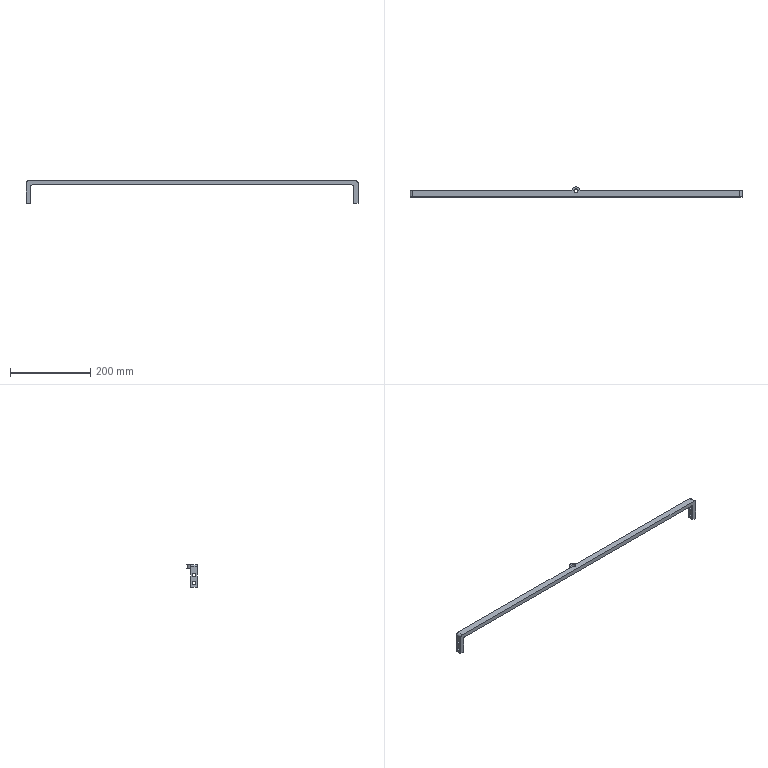Part | SolidWorks | features ICE 2, Extrusion 1, Fillet 1 | 1 solid | 26 faces | box 825 x 25 x 55 mm | volume 136025 mm3 | cylinder 15 | plane 11 | commonest cylinder face diameters 8 x8 10 x6 20 x1
STEP:
#1=CARTESIAN_POINT('',(-402.5,-7.5,-19.));
#2=VERTEX_POINT('',#1);
#3=CARTESIAN_POINT('',(-402.5,-7.5,-11.));
#4=VERTEX_POINT('',#3);
#5=CARTESIAN_POINT('',(-402.5,-7.5,-15.));
#6=DIRECTION('',(-1.,0.,0.));
#7=DIRECTION('',(0.,0.,1.));
#8=AXIS2_PLACEMENT_3D('',#5,#6,#7);
#9=CIRCLE('',#8,4.);
#10=EDGE_CURVE('',#2,#4,#9,.T.);
#11=ORIENTED_EDGE('',*,*,#10,.F.);
#12=CARTESIAN_POINT('',(-412.5,-7.5,-19.));
#13=VERTEX_POINT('',#12);
#14=CARTESIAN_POINT('',(-402.5,-7.5,-19.));
#15=DIRECTION('',(-1.,0.,0.));
#16=VECTOR('',#15,1000.);
#17=LINE('',#14,#16);
#18=EDGE_CURVE('',#2,#13,#17,.T.);
#19=ORIENTED_EDGE('',*,*,#18,.T.);
#20=CARTESIAN_POINT('',(-412.5,-7.5,-11.));
#21=VERTEX_POINT('',#20);
#22=CARTESIAN_POINT('',(-412.5,-7.5,-15.));
#23=DIRECTION('',(-1.,0.,0.));
#24=DIRECTION('',(0.,0.,1.));
#25=AXIS2_PLACEMENT_3D('',#22,#23,#24);
#26=CIRCLE('',#25,4.);
#27=EDGE_CURVE('',#13,#21,#26,.T.);
#28=ORIENTED_EDGE('',*,*,#27,.T.);
#29=CARTESIAN_POINT('',(-402.5,-7.5,-11.));
#30=DIRECTION('',(-1.,0.,0.));
#31=VECTOR('',#30,1000.);
#32=LINE('',#29,#31);
#33=EDGE_CURVE('',#4,#21,#32,.T.);
#34=ORIENTED_EDGE('',*,*,#33,.F.);
#35=EDGE_LOOP('',(#11,#19,#28,#34));
#36=FACE_OUTER_BOUND('',#35,.T.);
#37=CARTESIAN_POINT('',(-402.5,-7.5,-15.));
#38=DIRECTION('',(-1.,0.,0.));
#39=DIRECTION('',(0.,0.,1.));
#40=AXIS2_PLACEMENT_3D('',#37,#38,#39);
#41=CYLINDRICAL_SURFACE('',#40,4.);
#42=ADVANCED_FACE('',(#36),#41,.F.);
#43=CARTESIAN_POINT('',(-402.5,-7.5,-39.));
#44=VERTEX_POINT('',#43);
#45=CARTESIAN_POINT('',(-402.5,-7.5,-31.));
#46=VERTEX_POINT('',#45);
#47=CARTESIAN_POINT('',(-402.5,-7.5,-35.));
#48=DIRECTION('',(-1.,0.,0.));
#49=DIRECTION('',(0.,0.,1.));
#50=AXIS2_PLACEMENT_3D('',#47,#48,#49);
#51=CIRCLE('',#50,4.);
#52=EDGE_CURVE('',#44,#46,#51,.T.);
#53=ORIENTED_EDGE('',*,*,#52,.F.);
#54=CARTESIAN_POINT('',(-412.5,-7.5,-39.));
#55=VERTEX_POINT('',#54);
#56=CARTESIAN_POINT('',(-402.5,-7.5,-39.));
#57=DIRECTION('',(-1.,0.,0.));
#58=VECTOR('',#57,1000.);
#59=LINE('',#56,#58);
#60=EDGE_CURVE('',#44,#55,#59,.T.);
#61=ORIENTED_EDGE('',*,*,#60,.T.);
#62=CARTESIAN_POINT('',(-412.5,-7.5,-31.));
#63=VERTEX_POINT('',#62);
#64=CARTESIAN_POINT('',(-412.5,-7.5,-35.));
#65=DIRECTION('',(-1.,0.,0.));
#66=DIRECTION('',(0.,0.,1.));
#67=AXIS2_PLACEMENT_3D('',#64,#65,#66);
#68=CIRCLE('',#67,4.);
#69=EDGE_CURVE('',#55,#63,#68,.T.);
#70=ORIENTED_EDGE('',*,*,#69,.T.);
#71=CARTESIAN_POINT('',(-402.5,-7.5,-31.));
#72=DIRECTION('',(-1.,0.,0.));
#73=VECTOR('',#72,1000.);
#74=LINE('',#71,#73);
#75=EDGE_CURVE('',#46,#63,#74,.T.);
#76=ORIENTED_EDGE('',*,*,#75,.F.);
#77=EDGE_LOOP('',(#53,#61,#70,#76));
#78=FACE_OUTER_BOUND('',#77,.T.);
#79=CARTESIAN_POINT('',(-402.5,-7.5,-35.));
#80=DIRECTION('',(-1.,0.,0.));
#81=DIRECTION('',(0.,0.,1.));
#82=AXIS2_PLACEMENT_3D('',#79,#80,#81);
#83=CYLINDRICAL_SURFACE('',#82,4.);
#84=ADVANCED_FACE('',(#78),#83,.F.);
#85=CARTESIAN_POINT('',(402.5,-7.5,-31.));
#86=VERTEX_POINT('',#85);
#87=CARTESIAN_POINT('',(402.5,-7.5,-39.));
#88=VERTEX_POINT('',#87);
#89=CARTESIAN_POINT('',(402.5,-7.5,-35.));
#90=DIRECTION('',(1.,0.,0.));
#91=DIRECTION('',(0.,0.,-1.));
#92=AXIS2_PLACEMENT_3D('',#89,#90,#91);
#93=CIRCLE('',#92,4.);
#94=EDGE_CURVE('',#86,#88,#93,.T.);
#95=ORIENTED_EDGE('',*,*,#94,.F.);
#96=CARTESIAN_POINT('',(412.5,-7.5,-31.));
#97=VERTEX_POINT('',#96);
#98=CARTESIAN_POINT('',(402.5,-7.5,-31.));
#99=DIRECTION('',(1.,0.,0.));
#100=VECTOR('',#99,1000.);
#101=LINE('',#98,#100);
#102=EDGE_CURVE('',#86,#97,#101,.T.);
#103=ORIENTED_EDGE('',*,*,#102,.T.);
#104=CARTESIAN_POINT('',(412.5,-7.5,-39.));
#105=VERTEX_POINT('',#104);
#106=CARTESIAN_POINT('',(412.5,-7.5,-35.));
#107=DIRECTION('',(1.,0.,0.));
#108=DIRECTION('',(0.,0.,-1.));
#109=AXIS2_PLACEMENT_3D('',#106,#107,#108);
#110=CIRCLE('',#109,4.);
#111=EDGE_CURVE('',#97,#105,#110,.T.);
#112=ORIENTED_EDGE('',*,*,#111,.T.);
#113=CARTESIAN_POINT('',(402.5,-7.5,-39.));
#114=DIRECTION('',(1.,0.,0.));
#115=VECTOR('',#114,1000.);
#116=LINE('',#113,#115);
#117=EDGE_CURVE('',#88,#105,#116,.T.);
#118=ORIENTED_EDGE('',*,*,#117,.F.);
#119=EDGE_LOOP('',(#95,#103,#112,#118));
#120=FACE_OUTER_BOUND('',#119,.T.);
#121=CARTESIAN_POINT('',(402.5,-7.5,-35.));
#122=DIRECTION('',(1.,0.,0.));
#123=DIRECTION('',(0.,0.,-1.));
#124=AXIS2_PLACEMENT_3D('',#121,#122,#123);
#125=CYLINDRICAL_SURFACE('',#124,4.);
#126=ADVANCED_FACE('',(#120),#125,.F.);
#127=CARTESIAN_POINT('',(402.5,-7.5,-11.));
#128=VERTEX_POINT('',#127);
#129=CARTESIAN_POINT('',(402.5,-7.5,-19.));
#130=VERTEX_POINT('',#129);
#131=CARTESIAN_POINT('',(402.5,-7.5,-15.));
#132=DIRECTION('',(1.,0.,0.));
#133=DIRECTION('',(0.,0.,-1.));
#134=AXIS2_PLACEMENT_3D('',#131,#132,#133);
#135=CIRCLE('',#134,4.);
#136=EDGE_CURVE('',#128,#130,#135,.T.);
#137=ORIENTED_EDGE('',*,*,#136,.F.);
#138=CARTESIAN_POINT('',(412.5,-7.5,-11.));
#139=VERTEX_POINT('',#138);
#140=CARTESIAN_POINT('',(402.5,-7.5,-11.));
#141=DIRECTION('',(1.,0.,0.));
#142=VECTOR('',#141,1000.);
#143=LINE('',#140,#142);
#144=EDGE_CURVE('',#128,#139,#143,.T.);
#145=ORIENTED_EDGE('',*,*,#144,.T.);
#146=CARTESIAN_POINT('',(412.5,-7.5,-19.));
#147=VERTEX_POINT('',#146);
#148=CARTESIAN_POINT('',(412.5,-7.5,-15.));
#149=DIRECTION('',(1.,0.,0.));
#150=DIRECTION('',(0.,0.,-1.));
#151=AXIS2_PLACEMENT_3D('',#148,#149,#150);
#152=CIRCLE('',#151,4.);
#153=EDGE_CURVE('',#139,#147,#152,.T.);
#154=ORIENTED_EDGE('',*,*,#153,.T.);
#155=CARTESIAN_POINT('',(402.5,-7.5,-19.));
#156=DIRECTION('',(1.,0.,0.));
#157=VECTOR('',#156,1000.);
#158=LINE('',#155,#157);
#159=EDGE_CURVE('',#130,#147,#158,.T.);
#160=ORIENTED_EDGE('',*,*,#159,.F.);
#161=EDGE_LOOP('',(#137,#145,#154,#160));
#162=FACE_OUTER_BOUND('',#161,.T.);
#163=CARTESIAN_POINT('',(402.5,-7.5,-15.));
#164=DIRECTION('',(1.,0.,0.));
#165=DIRECTION('',(0.,0.,-1.));
#166=AXIS2_PLACEMENT_3D('',#163,#164,#165);
#167=CYLINDRICAL_SURFACE('',#166,4.);
#168=ADVANCED_FACE('',(#162),#167,.F.);
#169=CARTESIAN_POINT('',(-5.,0.,10.));
#170=VERTEX_POINT('',#169);
#171=CARTESIAN_POINT('',(5.,0.,10.));
#172=VERTEX_POINT('',#171);
#173=CARTESIAN_POINT('',(0.,0.,10.));
#174=DIRECTION('',(0.,0.,1.));
#175=DIRECTION('',(1.,0.,0.));
#176=AXIS2_PLACEMENT_3D('',#173,#174,#175);
#177=CIRCLE('',#176,5.);
#178=EDGE_CURVE('',#170,#172,#177,.T.);
#179=ORIENTED_EDGE('',*,*,#178,.T.);
#180=CARTESIAN_POINT('',(5.,0.,0.));
#181=VERTEX_POINT('',#180);
#182=CARTESIAN_POINT('',(5.,0.,10.));
#183=DIRECTION('',(0.,0.,-1.));
#184=VECTOR('',#183,1000.);
#185=LINE('',#182,#184);
#186=EDGE_CURVE('',#172,#181,#185,.T.);
#187=ORIENTED_EDGE('',*,*,#186,.T.);
#188=CARTESIAN_POINT('',(-5.,0.,0.));
#189=VERTEX_POINT('',#188);
#190=CARTESIAN_POINT('',(0.,0.,0.));
#191=DIRECTION('',(0.,0.,1.));
#192=DIRECTION('',(1.,0.,0.));
#193=AXIS2_PLACEMENT_3D('',#190,#191,#192);
#194=CIRCLE('',#193,5.);
#195=EDGE_CURVE('',#189,#181,#194,.T.);
#196=ORIENTED_EDGE('',*,*,#195,.F.);
#197=CARTESIAN_POINT('',(-5.,0.,10.));
#198=DIRECTION('',(0.,0.,-1.));
#199=VECTOR('',#198,1000.);
#200=LINE('',#197,#199);
#201=EDGE_CURVE('',#170,#189,#200,.T.);
#202=ORIENTED_EDGE('',*,*,#201,.F.);
#203=EDGE_LOOP('',(#179,#187,#196,#202));
#204=FACE_OUTER_BOUND('',#203,.T.);
#205=CARTESIAN_POINT('',(0.,0.,10.));
#206=DIRECTION('',(0.,0.,-1.));
#207=DIRECTION('',(-1.,0.,0.));
#208=AXIS2_PLACEMENT_3D('',#205,#206,#207);
#209=CYLINDRICAL_SURFACE('',#208,5.);
#210=ADVANCED_FACE('',(#204),#209,.F.);
#211=CARTESIAN_POINT('',(-10.,0.,10.));
#212=VERTEX_POINT('',#211);
#213=CARTESIAN_POINT('',(-407.5,0.,10.));
#214=VERTEX_POINT('',#213);
#215=CARTESIAN_POINT('',(-412.5,0.,10.));
#216=DIRECTION('',(-1.,0.,0.));
#217=VECTOR('',#216,1000.);
#218=LINE('',#215,#217);
#219=EDGE_CURVE('',#212,#214,#218,.T.);
#220=ORIENTED_EDGE('',*,*,#219,.T.);
#221=CARTESIAN_POINT('',(-407.5,-15.,10.));
#222=VERTEX_POINT('',#221);
#223=CARTESIAN_POINT('',(-407.5,-15.,10.));
#224=DIRECTION('',(0.,-1.,0.));
#225=VECTOR('',#224,1000.);
#226=LINE('',#223,#225);
#227=EDGE_CURVE('',#214,#222,#226,.T.);
#228=ORIENTED_EDGE('',*,*,#227,.T.);
#229=CARTESIAN_POINT('',(407.5,-15.,10.));
#230=VERTEX_POINT('',#229);
#231=CARTESIAN_POINT('',(0.,-15.,10.));
#232=DIRECTION('',(1.,0.,0.));
#233=VECTOR('',#232,1000.);
#234=LINE('',#231,#233);
#235=EDGE_CURVE('',#222,#230,#234,.T.);
#236=ORIENTED_EDGE('',*,*,#235,.T.);
#237=CARTESIAN_POINT('',(407.5,0.,10.));
#238=VERTEX_POINT('',#237);
#239=CARTESIAN_POINT('',(407.5,0.,10.));
#240=DIRECTION('',(0.,1.,0.));
#241=VECTOR('',#240,1000.);
#242=LINE('',#239,#241);
#243=EDGE_CURVE('',#230,#238,#242,.T.);
#244=ORIENTED_EDGE('',*,*,#243,.T.);
#245=CARTESIAN_POINT('',(10.,0.,10.));
#246=VERTEX_POINT('',#245);
#247=CARTESIAN_POINT('',(412.5,0.,10.));
#248=DIRECTION('',(-1.,0.,0.));
#249=VECTOR('',#248,1000.);
#250=LINE('',#247,#249);
#251=EDGE_CURVE('',#238,#246,#250,.T.);
#252=ORIENTED_EDGE('',*,*,#251,.T.);
#253=CARTESIAN_POINT('',(0.,0.,10.));
#254=DIRECTION('',(0.,0.,1.));
#255=DIRECTION('',(1.,0.,0.));
#256=AXIS2_PLACEMENT_3D('',#253,#254,#255);
#257=CIRCLE('',#256,10.);
#258=EDGE_CURVE('',#246,#212,#257,.T.);
#259=ORIENTED_EDGE('',*,*,#258,.T.);
#260=EDGE_LOOP('',(#220,#228,#236,#244,#252,#259));
#261=FACE_OUTER_BOUND('',#260,.T.);
#262=ORIENTED_EDGE('',*,*,#178,.F.);
#263=CARTESIAN_POINT('',(0.,0.,10.));
#264=DIRECTION('',(0.,0.,1.));
#265=DIRECTION('',(1.,0.,0.));
#266=AXIS2_PLACEMENT_3D('',#263,#264,#265);
#267=CIRCLE('',#266,5.);
#268=EDGE_CURVE('',#172,#170,#267,.T.);
#269=ORIENTED_EDGE('',*,*,#268,.F.);
#270=EDGE_LOOP('',(#262,#269));
#271=FACE_BOUND('',#270,.T.);
#272=CARTESIAN_POINT('',(0.,0.,10.));
#273=DIRECTION('',(0.,0.,1.));
#274=DIRECTION('',(1.,0.,0.));
#275=AXIS2_PLACEMENT_3D('',#272,#273,#274);
#276=PLANE('',#275);
#277=ADVANCED_FACE('',(#261,#271),#276,.T.);
#278=CARTESIAN_POINT('',(397.5,0.,0.));
#279=VERTEX_POINT('',#278);
#280=CARTESIAN_POINT('',(10.,0.,0.));
#281=VERTEX_POINT('',#280);
#282=CARTESIAN_POINT('',(412.5,0.,0.));
#283=DIRECTION('',(-1.,0.,0.));
#284=VECTOR('',#283,1000.);
#285=LINE('',#282,#284);
#286=EDGE_CURVE('',#279,#281,#285,.T.);
#287=ORIENTED_EDGE('',*,*,#286,.F.);
#288=CARTESIAN_POINT('',(397.5,-15.,0.));
#289=VERTEX_POINT('',#288);
#290=CARTESIAN_POINT('',(397.5,-15.,0.));
#291=DIRECTION('',(0.,-1.,0.));
#292=VECTOR('',#291,1000.);
#293=LINE('',#290,#292);
#294=EDGE_CURVE('',#279,#289,#293,.T.);
#295=ORIENTED_EDGE('',*,*,#294,.T.);
#296=CARTESIAN_POINT('',(-397.5,-15.,0.));
#297=VERTEX_POINT('',#296);
#298=CARTESIAN_POINT('',(0.,-15.,0.));
#299=DIRECTION('',(1.,0.,0.));
#300=VECTOR('',#299,1000.);
#301=LINE('',#298,#300);
#302=EDGE_CURVE('',#297,#289,#301,.T.);
#303=ORIENTED_EDGE('',*,*,#302,.F.);
#304=CARTESIAN_POINT('',(-397.5,0.,0.));
#305=VERTEX_POINT('',#304);
#306=CARTESIAN_POINT('',(-397.5,0.,0.));
#307=DIRECTION('',(0.,1.,0.));
#308=VECTOR('',#307,1000.);
#309=LINE('',#306,#308);
#310=EDGE_CURVE('',#297,#305,#309,.T.);
#311=ORIENTED_EDGE('',*,*,#310,.T.);
#312=CARTESIAN_POINT('',(-10.,0.,0.));
#313=VERTEX_POINT('',#312);
#314=CARTESIAN_POINT('',(-412.5,0.,0.));
#315=DIRECTION('',(-1.,0.,0.));
#316=VECTOR('',#315,1000.);
#317=LINE('',#314,#316);
#318=EDGE_CURVE('',#313,#305,#317,.T.);
#319=ORIENTED_EDGE('',*,*,#318,.F.);
#320=CARTESIAN_POINT('',(0.,0.,0.));
#321=DIRECTION('',(0.,0.,1.));
#322=DIRECTION('',(1.,0.,0.));
#323=AXIS2_PLACEMENT_3D('',#320,#321,#322);
#324=CIRCLE('',#323,10.);
#325=EDGE_CURVE('',#281,#313,#324,.T.);
#326=ORIENTED_EDGE('',*,*,#325,.F.);
#327=EDGE_LOOP('',(#287,#295,#303,#311,#319,#326));
#328=FACE_OUTER_BOUND('',#327,.T.);
#329=ORIENTED_EDGE('',*,*,#195,.T.);
#330=CARTESIAN_POINT('',(0.,0.,0.));
#331=DIRECTION('',(0.,0.,1.));
#332=DIRECTION('',(1.,0.,0.));
#333=AXIS2_PLACEMENT_3D('',#330,#331,#332);
#334=CIRCLE('',#333,5.);
#335=EDGE_CURVE('',#181,#189,#334,.T.);
#336=ORIENTED_EDGE('',*,*,#335,.T.);
#337=EDGE_LOOP('',(#329,#336));
#338=FACE_BOUND('',#337,.T.);
#339=CARTESIAN_POINT('',(0.,0.,0.));
#340=DIRECTION('',(0.,0.,1.));
#341=DIRECTION('',(1.,0.,0.));
#342=AXIS2_PLACEMENT_3D('',#339,#340,#341);
#343=PLANE('',#342);
#344=ADVANCED_FACE('',(#328,#338),#343,.F.);
#345=ORIENTED_EDGE('',*,*,#251,.F.);
#346=CARTESIAN_POINT('',(412.5,0.,5.));
#347=VERTEX_POINT('',#346);
#348=CARTESIAN_POINT('',(407.5,0.,5.));
#349=DIRECTION('',(0.,1.,0.));
#350=DIRECTION('',(0.,0.,-1.));
#351=AXIS2_PLACEMENT_3D('',#348,#349,#350);
#352=CIRCLE('',#351,5.);
#353=EDGE_CURVE('',#238,#347,#352,.T.);
#354=ORIENTED_EDGE('',*,*,#353,.T.);
#355=CARTESIAN_POINT('',(412.5,0.,-45.));
#356=VERTEX_POINT('',#355);
#357=CARTESIAN_POINT('',(412.5,0.,10.));
#358=DIRECTION('',(0.,0.,-1.));
#359=VECTOR('',#358,1000.);
#360=LINE('',#357,#359);
#361=EDGE_CURVE('',#347,#356,#360,.T.);
#362=ORIENTED_EDGE('',*,*,#361,.T.);
#363=CARTESIAN_POINT('',(402.5,0.,-45.));
#364=VERTEX_POINT('',#363);
#365=CARTESIAN_POINT('',(402.5,0.,-45.));
#366=DIRECTION('',(1.,0.,0.));
#367=VECTOR('',#366,1000.);
#368=LINE('',#365,#367);
#369=EDGE_CURVE('',#364,#356,#368,.T.);
#370=ORIENTED_EDGE('',*,*,#369,.F.);
#371=CARTESIAN_POINT('',(402.5,0.,-5.));
#372=VERTEX_POINT('',#371);
#373=CARTESIAN_POINT('',(402.5,0.,0.));
#374=DIRECTION('',(0.,0.,1.));
#375=VECTOR('',#374,1000.);
#376=LINE('',#373,#375);
#377=EDGE_CURVE('',#364,#372,#376,.T.);
#378=ORIENTED_EDGE('',*,*,#377,.T.);
#379=CARTESIAN_POINT('',(397.5,0.,-5.));
#380=DIRECTION('',(0.,-1.,0.));
#381=DIRECTION('',(0.,0.,-1.));
#382=AXIS2_PLACEMENT_3D('',#379,#380,#381);
#383=CIRCLE('',#382,5.);
#384=EDGE_CURVE('',#372,#279,#383,.T.);
#385=ORIENTED_EDGE('',*,*,#384,.T.);
#386=ORIENTED_EDGE('',*,*,#286,.T.);
#387=CARTESIAN_POINT('',(10.,0.,10.));
#388=DIRECTION('',(0.,0.,-1.));
#389=VECTOR('',#388,1000.);
#390=LINE('',#387,#389);
#391=EDGE_CURVE('',#246,#281,#390,.T.);
#392=ORIENTED_EDGE('',*,*,#391,.F.);
#393=EDGE_LOOP('',(#345,#354,#362,#370,#378,#385,#386,#392));
#394=FACE_OUTER_BOUND('',#393,.T.);
#395=CARTESIAN_POINT('',(412.5,0.,10.));
#396=DIRECTION('',(0.,-1.,0.));
#397=DIRECTION('',(0.,0.,-1.));
#398=AXIS2_PLACEMENT_3D('',#395,#396,#397);
#399=PLANE('',#398);
#400=ADVANCED_FACE('',(#394),#399,.F.);
#401=ORIENTED_EDGE('',*,*,#325,.T.);
#402=CARTESIAN_POINT('',(-10.,0.,10.));
#403=DIRECTION('',(0.,0.,-1.));
#404=VECTOR('',#403,1000.);
#405=LINE('',#402,#404);
#406=EDGE_CURVE('',#212,#313,#405,.T.);
#407=ORIENTED_EDGE('',*,*,#406,.F.);
#408=ORIENTED_EDGE('',*,*,#258,.F.);
#409=ORIENTED_EDGE('',*,*,#391,.T.);
#410=EDGE_LOOP('',(#401,#407,#408,#409));
#411=FACE_OUTER_BOUND('',#410,.T.);
#412=CARTESIAN_POINT('',(0.,0.,10.));
#413=DIRECTION('',(0.,0.,-1.));
#414=DIRECTION('',(-1.,0.,0.));
#415=AXIS2_PLACEMENT_3D('',#412,#413,#414);
#416=CYLINDRICAL_SURFACE('',#415,10.);
#417=ADVANCED_FACE('',(#411),#416,.T.);
#418=CARTESIAN_POINT('',(-412.5,0.,5.));
#419=VERTEX_POINT('',#418);
#420=CARTESIAN_POINT('',(-412.5,0.,-45.));
#421=VERTEX_POINT('',#420);
#422=CARTESIAN_POINT('',(-412.5,0.,10.));
#423=DIRECTION('',(0.,0.,-1.));
#424=VECTOR('',#423,1000.);
#425=LINE('',#422,#424);
#426=EDGE_CURVE('',#419,#421,#425,.T.);
#427=ORIENTED_EDGE('',*,*,#426,.F.);
#428=CARTESIAN_POINT('',(-407.5,0.,5.));
#429=DIRECTION('',(0.,1.,0.));
#430=DIRECTION('',(0.,0.,-1.));
#431=AXIS2_PLACEMENT_3D('',#428,#429,#430);
#432=CIRCLE('',#431,5.);
#433=EDGE_CURVE('',#419,#214,#432,.T.);
#434=ORIENTED_EDGE('',*,*,#433,.T.);
#435=ORIENTED_EDGE('',*,*,#219,.F.);
#436=ORIENTED_EDGE('',*,*,#406,.T.);
#437=ORIENTED_EDGE('',*,*,#318,.T.);
#438=CARTESIAN_POINT('',(-402.5,0.,-5.));
#439=VERTEX_POINT('',#438);
#440=CARTESIAN_POINT('',(-397.5,0.,-5.));
#441=DIRECTION('',(0.,-1.,0.));
#442=DIRECTION('',(0.,0.,-1.));
#443=AXIS2_PLACEMENT_3D('',#440,#441,#442);
#444=CIRCLE('',#443,5.);
#445=EDGE_CURVE('',#305,#439,#444,.T.);
#446=ORIENTED_EDGE('',*,*,#445,.T.);
#447=CARTESIAN_POINT('',(-402.5,0.,-45.));
#448=VERTEX_POINT('',#447);
#449=CARTESIAN_POINT('',(-402.5,0.,0.));
#450=DIRECTION('',(0.,0.,-1.));
#451=VECTOR('',#450,1000.);
#452=LINE('',#449,#451);
#453=EDGE_CURVE('',#439,#448,#452,.T.);
#454=ORIENTED_EDGE('',*,*,#453,.T.);
#455=CARTESIAN_POINT('',(-402.5,0.,-45.));
#456=DIRECTION('',(-1.,0.,0.));
#457=VECTOR('',#456,1000.);
#458=LINE('',#455,#457);
#459=EDGE_CURVE('',#448,#421,#458,.T.);
#460=ORIENTED_EDGE('',*,*,#459,.T.);
#461=EDGE_LOOP('',(#427,#434,#435,#436,#437,#446,#454,#460));
#462=FACE_OUTER_BOUND('',#461,.T.);
#463=CARTESIAN_POINT('',(-412.5,0.,10.));
#464=DIRECTION('',(0.,-1.,0.));
#465=DIRECTION('',(0.,0.,-1.));
#466=AXIS2_PLACEMENT_3D('',#463,#464,#465);
#467=PLANE('',#466);
#468=ADVANCED_FACE('',(#462),#467,.F.);
#469=CARTESIAN_POINT('',(-412.5,-15.,5.));
#470=VERTEX_POINT('',#469);
#471=CARTESIAN_POINT('',(-412.5,-15.,-45.));
#472=VERTEX_POINT('',#471);
#473=CARTESIAN_POINT('',(-412.5,-15.,10.));
#474=DIRECTION('',(0.,0.,-1.));
#475=VECTOR('',#474,1000.);
#476=LINE('',#473,#475);
#477=EDGE_CURVE('',#470,#472,#476,.T.);
#478=ORIENTED_EDGE('',*,*,#477,.F.);
#479=CARTESIAN_POINT('',(-412.5,0.,5.));
#480=DIRECTION('',(0.,1.,0.));
#481=VECTOR('',#480,1000.);
#482=LINE('',#479,#481);
#483=EDGE_CURVE('',#470,#419,#482,.T.);
#484=ORIENTED_EDGE('',*,*,#483,.T.);
#485=ORIENTED_EDGE('',*,*,#426,.T.);
#486=CARTESIAN_POINT('',(-412.5,0.,-45.));
#487=DIRECTION('',(0.,-1.,0.));
#488=VECTOR('',#487,1000.);
#489=LINE('',#486,#488);
#490=EDGE_CURVE('',#421,#472,#489,.T.);
#491=ORIENTED_EDGE('',*,*,#490,.T.);
#492=EDGE_LOOP('',(#478,#484,#485,#491));
#493=FACE_OUTER_BOUND('',#492,.T.);
#494=CARTESIAN_POINT('',(-412.5,-7.5,-15.));
#495=DIRECTION('',(-1.,0.,0.));
#496=DIRECTION('',(0.,0.,1.));
#497=AXIS2_PLACEMENT_3D('',#494,#495,#496);
#498=CIRCLE('',#497,4.);
#499=EDGE_CURVE('',#21,#13,#498,.T.);
#500=ORIENTED_EDGE('',*,*,#499,.F.);
#501=ORIENTED_EDGE('',*,*,#27,.F.);
#502=EDGE_LOOP('',(#500,#501));
#503=FACE_BOUND('',#502,.T.);
#504=CARTESIAN_POINT('',(-412.5,-7.5,-35.));
#505=DIRECTION('',(-1.,0.,0.));
#506=DIRECTION('',(0.,0.,1.));
#507=AXIS2_PLACEMENT_3D('',#504,#505,#506);
#508=CIRCLE('',#507,4.);
#509=EDGE_CURVE('',#63,#55,#508,.T.);
#510=ORIENTED_EDGE('',*,*,#509,.F.);
#511=ORIENTED_EDGE('',*,*,#69,.F.);
#512=EDGE_LOOP('',(#510,#511));
#513=FACE_BOUND('',#512,.T.);
#514=CARTESIAN_POINT('',(-412.5,-15.,10.));
#515=DIRECTION('',(1.,0.,0.));
#516=DIRECTION('',(0.,0.,-1.));
#517=AXIS2_PLACEMENT_3D('',#514,#515,#516);
#518=PLANE('',#517);
#519=ADVANCED_FACE('',(#493,#503,#513),#518,.F.);
#520=ORIENTED_EDGE('',*,*,#235,.F.);
#521=CARTESIAN_POINT('',(-407.5,-15.,5.));
#522=DIRECTION('',(0.,-1.,0.));
#523=DIRECTION('',(0.,0.,1.));
#524=AXIS2_PLACEMENT_3D('',#521,#522,#523);
#525=CIRCLE('',#524,5.);
#526=EDGE_CURVE('',#222,#470,#525,.T.);
#527=ORIENTED_EDGE('',*,*,#526,.T.);
#528=ORIENTED_EDGE('',*,*,#477,.T.);
#529=CARTESIAN_POINT('',(-402.5,-15.,-45.));
#530=VERTEX_POINT('',#529);
#531=CARTESIAN_POINT('',(-402.5,-15.,-45.));
#532=DIRECTION('',(-1.,0.,0.));
#533=VECTOR('',#532,1000.);
#534=LINE('',#531,#533);
#535=EDGE_CURVE('',#530,#472,#534,.T.);
#536=ORIENTED_EDGE('',*,*,#535,.F.);
#537=CARTESIAN_POINT('',(-402.5,-15.,-5.));
#538=VERTEX_POINT('',#537);
#539=CARTESIAN_POINT('',(-402.5,-15.,0.));
#540=DIRECTION('',(0.,0.,1.));
#541=VECTOR('',#540,1000.);
#542=LINE('',#539,#541);
#543=EDGE_CURVE('',#530,#538,#542,.T.);
#544=ORIENTED_EDGE('',*,*,#543,.T.);
#545=CARTESIAN_POINT('',(-397.5,-15.,-5.));
#546=DIRECTION('',(0.,1.,0.));
#547=DIRECTION('',(0.,0.,1.));
#548=AXIS2_PLACEMENT_3D('',#545,#546,#547);
#549=CIRCLE('',#548,5.);
#550=EDGE_CURVE('',#538,#297,#549,.T.);
#551=ORIENTED_EDGE('',*,*,#550,.T.);
#552=ORIENTED_EDGE('',*,*,#302,.T.);
#553=CARTESIAN_POINT('',(402.5,-15.,-5.));
#554=VERTEX_POINT('',#553);
#555=CARTESIAN_POINT('',(397.5,-15.,-5.));
#556=DIRECTION('',(0.,1.,0.));
#557=DIRECTION('',(0.,0.,1.));
#558=AXIS2_PLACEMENT_3D('',#555,#556,#557);
#559=CIRCLE('',#558,5.);
#560=EDGE_CURVE('',#289,#554,#559,.T.);
#561=ORIENTED_EDGE('',*,*,#560,.T.);
#562=CARTESIAN_POINT('',(402.5,-15.,-45.));
#563=VERTEX_POINT('',#562);
#564=CARTESIAN_POINT('',(402.5,-15.,0.));
#565=DIRECTION('',(0.,0.,-1.));
#566=VECTOR('',#565,1000.);
#567=LINE('',#564,#566);
#568=EDGE_CURVE('',#554,#563,#567,.T.);
#569=ORIENTED_EDGE('',*,*,#568,.T.);
#570=CARTESIAN_POINT('',(412.5,-15.,-45.));
#571=VERTEX_POINT('',#570);
#572=CARTESIAN_POINT('',(402.5,-15.,-45.));
#573=DIRECTION('',(1.,0.,0.));
#574=VECTOR('',#573,1000.);
#575=LINE('',#572,#574);
#576=EDGE_CURVE('',#563,#571,#575,.T.);
#577=ORIENTED_EDGE('',*,*,#576,.T.);
#578=CARTESIAN_POINT('',(412.5,-15.,5.));
#579=VERTEX_POINT('',#578);
#580=CARTESIAN_POINT('',(412.5,-15.,10.));
#581=DIRECTION('',(0.,0.,-1.));
#582=VECTOR('',#581,1000.);
#583=LINE('',#580,#582);
#584=EDGE_CURVE('',#579,#571,#583,.T.);
#585=ORIENTED_EDGE('',*,*,#584,.F.);
#586=CARTESIAN_POINT('',(407.5,-15.,5.));
#587=DIRECTION('',(0.,-1.,0.));
#588=DIRECTION('',(0.,0.,1.));
#589=AXIS2_PLACEMENT_3D('',#586,#587,#588);
#590=CIRCLE('',#589,5.);
#591=EDGE_CURVE('',#579,#230,#590,.T.);
#592=ORIENTED_EDGE('',*,*,#591,.T.);
#593=EDGE_LOOP('',(#520,#527,#528,#536,#544,#551,#552,#561,#569,#577,#585,#592));
#594=FACE_OUTER_BOUND('',#593,.T.);
#595=CARTESIAN_POINT('',(0.,-15.,10.));
#596=DIRECTION('',(0.,1.,0.));
#597=DIRECTION('',(0.,0.,1.));
#598=AXIS2_PLACEMENT_3D('',#595,#596,#597);
#599=PLANE('',#598);
#600=ADVANCED_FACE('',(#594),#599,.F.);
#601=ORIENTED_EDGE('',*,*,#361,.F.);
#602=CARTESIAN_POINT('',(412.5,-15.,5.));
#603=DIRECTION('',(0.,-1.,0.));
#604=VECTOR('',#603,1000.);
#605=LINE('',#602,#604);
#606=EDGE_CURVE('',#347,#579,#605,.T.);
#607=ORIENTED_EDGE('',*,*,#606,.T.);
#608=ORIENTED_EDGE('',*,*,#584,.T.);
#609=CARTESIAN_POINT('',(412.5,0.,-45.));
#610=DIRECTION('',(0.,1.,0.));
#611=VECTOR('',#610,1000.);
#612=LINE('',#609,#611);
#613=EDGE_CURVE('',#571,#356,#612,.T.);
#614=ORIENTED_EDGE('',*,*,#613,.T.);
#615=EDGE_LOOP('',(#601,#607,#608,#614));
#616=FACE_OUTER_BOUND('',#615,.T.);
#617=CARTESIAN_POINT('',(412.5,-7.5,-35.));
#618=DIRECTION('',(1.,0.,0.));
#619=DIRECTION('',(0.,0.,-1.));
#620=AXIS2_PLACEMENT_3D('',#617,#618,#619);
#621=CIRCLE('',#620,4.);
#622=EDGE_CURVE('',#105,#97,#621,.T.);
#623=ORIENTED_EDGE('',*,*,#622,.F.);
#624=ORIENTED_EDGE('',*,*,#111,.F.);
#625=EDGE_LOOP('',(#623,#624));
#626=FACE_BOUND('',#625,.T.);
#627=CARTESIAN_POINT('',(412.5,-7.5,-15.));
#628=DIRECTION('',(1.,0.,0.));
#629=DIRECTION('',(0.,0.,-1.));
#630=AXIS2_PLACEMENT_3D('',#627,#628,#629);
#631=CIRCLE('',#630,4.);
#632=EDGE_CURVE('',#147,#139,#631,.T.);
#633=ORIENTED_EDGE('',*,*,#632,.F.);
#634=ORIENTED_EDGE('',*,*,#153,.F.);
#635=EDGE_LOOP('',(#633,#634));
#636=FACE_BOUND('',#635,.T.);
#637=CARTESIAN_POINT('',(412.5,-15.,10.));
#638=DIRECTION('',(-1.,0.,0.));
#639=DIRECTION('',(0.,0.,1.));
#640=AXIS2_PLACEMENT_3D('',#637,#638,#639);
#641=PLANE('',#640);
#642=ADVANCED_FACE('',(#616,#626,#636),#641,.F.);
#643=ORIENTED_EDGE('',*,*,#186,.F.);
#644=ORIENTED_EDGE('',*,*,#268,.T.);
#645=ORIENTED_EDGE('',*,*,#201,.T.);
#646=ORIENTED_EDGE('',*,*,#335,.F.);
#647=EDGE_LOOP('',(#643,#644,#645,#646));
#648=FACE_OUTER_BOUND('',#647,.T.);
#649=CARTESIAN_POINT('',(0.,0.,10.));
#650=DIRECTION('',(0.,0.,-1.));
#651=DIRECTION('',(-1.,0.,0.));
#652=AXIS2_PLACEMENT_3D('',#649,#650,#651);
#653=CYLINDRICAL_SURFACE('',#652,5.);
#654=ADVANCED_FACE('',(#648),#653,.F.);
#655=ORIENTED_EDGE('',*,*,#613,.F.);
#656=ORIENTED_EDGE('',*,*,#576,.F.);
#657=CARTESIAN_POINT('',(402.5,0.,-45.));
#658=DIRECTION('',(0.,1.,0.));
#659=VECTOR('',#658,1000.);
#660=LINE('',#657,#659);
#661=EDGE_CURVE('',#563,#364,#660,.T.);
#662=ORIENTED_EDGE('',*,*,#661,.T.);
#663=ORIENTED_EDGE('',*,*,#369,.T.);
#664=EDGE_LOOP('',(#655,#656,#662,#663));
#665=FACE_OUTER_BOUND('',#664,.T.);
#666=CARTESIAN_POINT('',(402.5,0.,-45.));
#667=DIRECTION('',(0.,0.,-1.));
#668=DIRECTION('',(-1.,0.,0.));
#669=AXIS2_PLACEMENT_3D('',#666,#667,#668);
#670=PLANE('',#669);
#671=ADVANCED_FACE('',(#665),#670,.T.);
#672=CARTESIAN_POINT('',(402.5,-7.5,-35.));
#673=DIRECTION('',(1.,0.,0.));
#674=DIRECTION('',(0.,0.,-1.));
#675=AXIS2_PLACEMENT_3D('',#672,#673,#674);
#676=CIRCLE('',#675,4.);
#677=EDGE_CURVE('',#88,#86,#676,.T.);
#678=ORIENTED_EDGE('',*,*,#677,.T.);
#679=ORIENTED_EDGE('',*,*,#94,.T.);
#680=EDGE_LOOP('',(#678,#679));
#681=FACE_BOUND('',#680,.T.);
#682=CARTESIAN_POINT('',(402.5,-7.5,-15.));
#683=DIRECTION('',(1.,0.,0.));
#684=DIRECTION('',(0.,0.,-1.));
#685=AXIS2_PLACEMENT_3D('',#682,#683,#684);
#686=CIRCLE('',#685,4.);
#687=EDGE_CURVE('',#130,#128,#686,.T.);
#688=ORIENTED_EDGE('',*,*,#687,.T.);
#689=ORIENTED_EDGE('',*,*,#136,.T.);
#690=EDGE_LOOP('',(#688,#689));
#691=FACE_BOUND('',#690,.T.);
#692=ORIENTED_EDGE('',*,*,#568,.F.);
#693=CARTESIAN_POINT('',(402.5,0.,-5.));
#694=DIRECTION('',(0.,1.,0.));
#695=VECTOR('',#694,1000.);
#696=LINE('',#693,#695);
#697=EDGE_CURVE('',#554,#372,#696,.T.);
#698=ORIENTED_EDGE('',*,*,#697,.T.);
#699=ORIENTED_EDGE('',*,*,#377,.F.);
#700=ORIENTED_EDGE('',*,*,#661,.F.);
#701=EDGE_LOOP('',(#692,#698,#699,#700));
#702=FACE_OUTER_BOUND('',#701,.T.);
#703=CARTESIAN_POINT('',(402.5,0.,0.));
#704=DIRECTION('',(1.,0.,0.));
#705=DIRECTION('',(0.,0.,-1.));
#706=AXIS2_PLACEMENT_3D('',#703,#704,#705);
#707=PLANE('',#706);
#708=ADVANCED_FACE('',(#681,#691,#702),#707,.F.);
#709=ORIENTED_EDGE('',*,*,#144,.F.);
#710=ORIENTED_EDGE('',*,*,#687,.F.);
#711=ORIENTED_EDGE('',*,*,#159,.T.);
#712=ORIENTED_EDGE('',*,*,#632,.T.);
#713=EDGE_LOOP('',(#709,#710,#711,#712));
#714=FACE_OUTER_BOUND('',#713,.T.);
#715=CARTESIAN_POINT('',(402.5,-7.5,-15.));
#716=DIRECTION('',(1.,0.,0.));
#717=DIRECTION('',(0.,0.,-1.));
#718=AXIS2_PLACEMENT_3D('',#715,#716,#717);
#719=CYLINDRICAL_SURFACE('',#718,4.);
#720=ADVANCED_FACE('',(#714),#719,.F.);
#721=ORIENTED_EDGE('',*,*,#102,.F.);
#722=ORIENTED_EDGE('',*,*,#677,.F.);
#723=ORIENTED_EDGE('',*,*,#117,.T.);
#724=ORIENTED_EDGE('',*,*,#622,.T.);
#725=EDGE_LOOP('',(#721,#722,#723,#724));
#726=FACE_OUTER_BOUND('',#725,.T.);
#727=CARTESIAN_POINT('',(402.5,-7.5,-35.));
#728=DIRECTION('',(1.,0.,0.));
#729=DIRECTION('',(0.,0.,-1.));
#730=AXIS2_PLACEMENT_3D('',#727,#728,#729);
#731=CYLINDRICAL_SURFACE('',#730,4.);
#732=ADVANCED_FACE('',(#726),#731,.F.);
#733=ORIENTED_EDGE('',*,*,#490,.F.);
#734=ORIENTED_EDGE('',*,*,#459,.F.);
#735=CARTESIAN_POINT('',(-402.5,0.,-45.));
#736=DIRECTION('',(0.,-1.,0.));
#737=VECTOR('',#736,1000.);
#738=LINE('',#735,#737);
#739=EDGE_CURVE('',#448,#530,#738,.T.);
#740=ORIENTED_EDGE('',*,*,#739,.T.);
#741=ORIENTED_EDGE('',*,*,#535,.T.);
#742=EDGE_LOOP('',(#733,#734,#740,#741));
#743=FACE_OUTER_BOUND('',#742,.T.);
#744=CARTESIAN_POINT('',(-402.5,0.,-45.));
#745=DIRECTION('',(0.,0.,-1.));
#746=DIRECTION('',(-1.,0.,0.));
#747=AXIS2_PLACEMENT_3D('',#744,#745,#746);
#748=PLANE('',#747);
#749=ADVANCED_FACE('',(#743),#748,.T.);
#750=CARTESIAN_POINT('',(-402.5,-7.5,-15.));
#751=DIRECTION('',(-1.,0.,0.));
#752=DIRECTION('',(0.,0.,1.));
#753=AXIS2_PLACEMENT_3D('',#750,#751,#752);
#754=CIRCLE('',#753,4.);
#755=EDGE_CURVE('',#4,#2,#754,.T.);
#756=ORIENTED_EDGE('',*,*,#755,.T.);
#757=ORIENTED_EDGE('',*,*,#10,.T.);
#758=EDGE_LOOP('',(#756,#757));
#759=FACE_BOUND('',#758,.T.);
#760=CARTESIAN_POINT('',(-402.5,-7.5,-35.));
#761=DIRECTION('',(-1.,0.,0.));
#762=DIRECTION('',(0.,0.,1.));
#763=AXIS2_PLACEMENT_3D('',#760,#761,#762);
#764=CIRCLE('',#763,4.);
#765=EDGE_CURVE('',#46,#44,#764,.T.);
#766=ORIENTED_EDGE('',*,*,#765,.T.);
#767=ORIENTED_EDGE('',*,*,#52,.T.);
#768=EDGE_LOOP('',(#766,#767));
#769=FACE_BOUND('',#768,.T.);
#770=ORIENTED_EDGE('',*,*,#453,.F.);
#771=CARTESIAN_POINT('',(-402.5,0.,-5.));
#772=DIRECTION('',(0.,-1.,0.));
#773=VECTOR('',#772,1000.);
#774=LINE('',#771,#773);
#775=EDGE_CURVE('',#439,#538,#774,.T.);
#776=ORIENTED_EDGE('',*,*,#775,.T.);
#777=ORIENTED_EDGE('',*,*,#543,.F.);
#778=ORIENTED_EDGE('',*,*,#739,.F.);
#779=EDGE_LOOP('',(#770,#776,#777,#778));
#780=FACE_OUTER_BOUND('',#779,.T.);
#781=CARTESIAN_POINT('',(-402.5,0.,0.));
#782=DIRECTION('',(1.,0.,0.));
#783=DIRECTION('',(0.,0.,-1.));
#784=AXIS2_PLACEMENT_3D('',#781,#782,#783);
#785=PLANE('',#784);
#786=ADVANCED_FACE('',(#759,#769,#780),#785,.T.);
#787=ORIENTED_EDGE('',*,*,#60,.F.);
#788=ORIENTED_EDGE('',*,*,#765,.F.);
#789=ORIENTED_EDGE('',*,*,#75,.T.);
#790=ORIENTED_EDGE('',*,*,#509,.T.);
#791=EDGE_LOOP('',(#787,#788,#789,#790));
#792=FACE_OUTER_BOUND('',#791,.T.);
#793=CARTESIAN_POINT('',(-402.5,-7.5,-35.));
#794=DIRECTION('',(-1.,0.,0.));
#795=DIRECTION('',(0.,0.,1.));
#796=AXIS2_PLACEMENT_3D('',#793,#794,#795);
#797=CYLINDRICAL_SURFACE('',#796,4.);
#798=ADVANCED_FACE('',(#792),#797,.F.);
#799=ORIENTED_EDGE('',*,*,#18,.F.);
#800=ORIENTED_EDGE('',*,*,#755,.F.);
#801=ORIENTED_EDGE('',*,*,#33,.T.);
#802=ORIENTED_EDGE('',*,*,#499,.T.);
#803=EDGE_LOOP('',(#799,#800,#801,#802));
#804=FACE_OUTER_BOUND('',#803,.T.);
#805=CARTESIAN_POINT('',(-402.5,-7.5,-15.));
#806=DIRECTION('',(-1.,0.,0.));
#807=DIRECTION('',(0.,0.,1.));
#808=AXIS2_PLACEMENT_3D('',#805,#806,#807);
#809=CYLINDRICAL_SURFACE('',#808,4.);
#810=ADVANCED_FACE('',(#804),#809,.F.);
#811=ORIENTED_EDGE('',*,*,#433,.F.);
#812=ORIENTED_EDGE('',*,*,#483,.F.);
#813=ORIENTED_EDGE('',*,*,#526,.F.);
#814=ORIENTED_EDGE('',*,*,#227,.F.);
#815=EDGE_LOOP('',(#811,#812,#813,#814));
#816=FACE_OUTER_BOUND('',#815,.T.);
#817=CARTESIAN_POINT('',(-407.5,0.,5.));
#818=DIRECTION('',(0.,1.,0.));
#819=DIRECTION('',(0.,0.,1.));
#820=AXIS2_PLACEMENT_3D('',#817,#818,#819);
#821=CYLINDRICAL_SURFACE('',#820,5.);
#822=ADVANCED_FACE('',(#816),#821,.T.);
#823=ORIENTED_EDGE('',*,*,#384,.F.);
#824=ORIENTED_EDGE('',*,*,#697,.F.);
#825=ORIENTED_EDGE('',*,*,#560,.F.);
#826=ORIENTED_EDGE('',*,*,#294,.F.);
#827=EDGE_LOOP('',(#823,#824,#825,#826));
#828=FACE_OUTER_BOUND('',#827,.T.);
#829=CARTESIAN_POINT('',(397.5,0.,-5.));
#830=DIRECTION('',(0.,1.,0.));
#831=DIRECTION('',(0.,0.,1.));
#832=AXIS2_PLACEMENT_3D('',#829,#830,#831);
#833=CYLINDRICAL_SURFACE('',#832,5.);
#834=ADVANCED_FACE('',(#828),#833,.F.);
#835=ORIENTED_EDGE('',*,*,#591,.F.);
#836=ORIENTED_EDGE('',*,*,#606,.F.);
#837=ORIENTED_EDGE('',*,*,#353,.F.);
#838=ORIENTED_EDGE('',*,*,#243,.F.);
#839=EDGE_LOOP('',(#835,#836,#837,#838));
#840=FACE_OUTER_BOUND('',#839,.T.);
#841=CARTESIAN_POINT('',(407.5,0.,5.));
#842=DIRECTION('',(0.,-1.,0.));
#843=DIRECTION('',(0.,0.,-1.));
#844=AXIS2_PLACEMENT_3D('',#841,#842,#843);
#845=CYLINDRICAL_SURFACE('',#844,5.);
#846=ADVANCED_FACE('',(#840),#845,.T.);
#847=ORIENTED_EDGE('',*,*,#550,.F.);
#848=ORIENTED_EDGE('',*,*,#775,.F.);
#849=ORIENTED_EDGE('',*,*,#445,.F.);
#850=ORIENTED_EDGE('',*,*,#310,.F.);
#851=EDGE_LOOP('',(#847,#848,#849,#850));
#852=FACE_OUTER_BOUND('',#851,.T.);
#853=CARTESIAN_POINT('',(-397.5,0.,-5.));
#854=DIRECTION('',(0.,1.,0.));
#855=DIRECTION('',(0.,0.,1.));
#856=AXIS2_PLACEMENT_3D('',#853,#854,#855);
#857=CYLINDRICAL_SURFACE('',#856,5.);
#858=ADVANCED_FACE('',(#852),#857,.F.);
#859=CLOSED_SHELL('',(#42,#84,#126,#168,#210,#277,#344,#400,#417,#468,#519,#600,#642,#654,#671,#708,#720,#732,#749,#786,#798,#810,#822,#834,#846,#858));
#860=MANIFOLD_SOLID_BREP('',#859);
#861=CARTESIAN_POINT('',(0.,0.,0.));
#862=DIRECTION('',(0.,0.,1.));
#863=DIRECTION('',(1.,0.,0.));
#864=AXIS2_PLACEMENT_3D('',#861,#862,#863);
#865=(LENGTH_UNIT()NAMED_UNIT(*)SI_UNIT(.MILLI.,.METRE.));
#866=UNCERTAINTY_MEASURE_WITH_UNIT(LENGTH_MEASURE(0.00001),#865,'','');
#867=(NAMED_UNIT(*)PLANE_ANGLE_UNIT()SI_UNIT($,.RADIAN.));
#868=(NAMED_UNIT(*)SI_UNIT($,.STERADIAN.)SOLID_ANGLE_UNIT());
#869=(GEOMETRIC_REPRESENTATION_CONTEXT(3)GLOBAL_UNCERTAINTY_ASSIGNED_CONTEXT((#866))GLOBAL_UNIT_ASSIGNED_CONTEXT((#865,#867,#868))REPRESENTATION_CONTEXT('',''));
#870=ADVANCED_BREP_SHAPE_REPRESENTATION('',(#860,#864),#869);